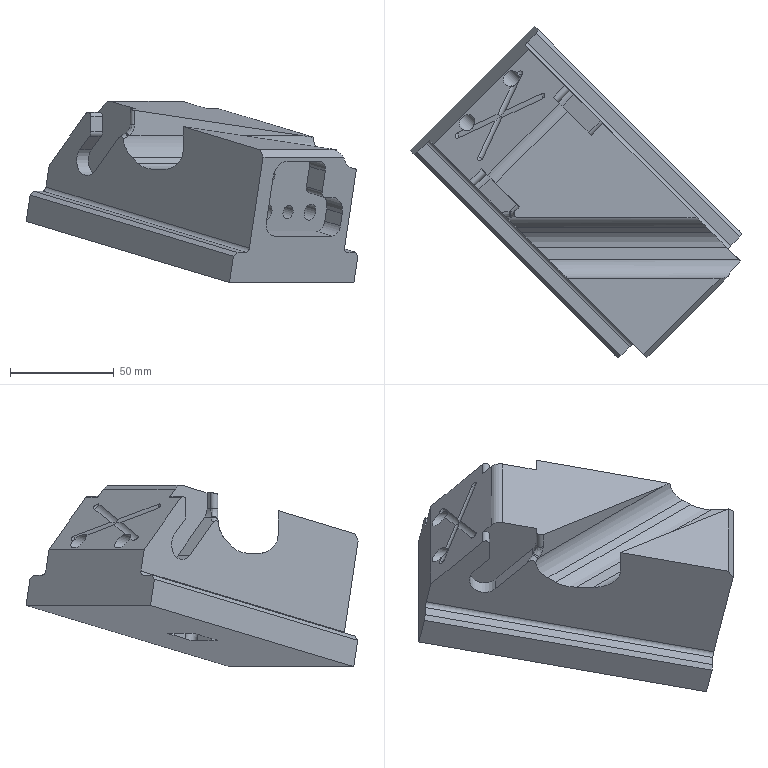Part | STEP file | gslz 2016.10.28-13_id94_x_t | 1 solid | 85 faces | box 160.23 x 160.363 x 87.521 mm | volume 526348 mm3 | plane 41 | cylinder 34 | sphere 4 | cone 3 | spline 3 | commonest cylinder face diameters 6 x11 4 x5 12 x3 6.8 x2 8 x2 10 x2